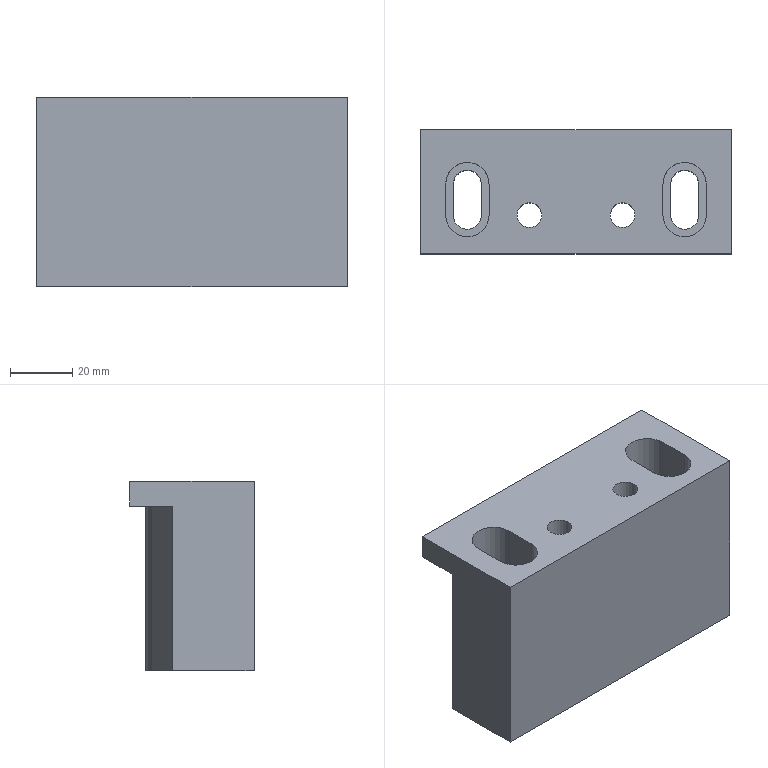Part | NX | features 1605158808 2 | 1 solid | 30 faces | box 100 x 40 x 61 mm | volume 179848 mm3 | plane 19 | cylinder 11 | commonest cylinder face diameters 9 x4 14 x4 8.001 x2 30 x1
STEP:
#1=CARTESIAN_POINT('',(-322.,-117.55,-2.5));
#2=VERTEX_POINT('',#1);
#3=CARTESIAN_POINT('',(-318.,-117.55,-2.5));
#4=DIRECTION('',(0.,0.,-1.));
#5=DIRECTION('',(-1.,0.,0.));
#6=AXIS2_PLACEMENT_3D('',#3,#4,#5);
#7=CIRCLE('',#6,4.);
#8=EDGE_CURVE('',#2,#2,#7,.T.);
#9=ORIENTED_EDGE('',*,*,#8,.F.);
#10=EDGE_LOOP('',(#9));
#11=FACE_BOUND('',#10,.T.);
#12=CARTESIAN_POINT('',(-352.,-117.55,-2.5));
#13=VERTEX_POINT('',#12);
#14=CARTESIAN_POINT('',(-348.,-117.55,-2.5));
#15=DIRECTION('',(0.,0.,-1.));
#16=DIRECTION('',(-1.,0.,0.));
#17=AXIS2_PLACEMENT_3D('',#14,#15,#16);
#18=CIRCLE('',#17,4.);
#19=EDGE_CURVE('',#13,#13,#18,.T.);
#20=ORIENTED_EDGE('',*,*,#19,.F.);
#21=EDGE_LOOP('',(#20));
#22=FACE_BOUND('',#21,.T.);
#23=CARTESIAN_POINT('',(-383.,-103.71,-2.5));
#24=VERTEX_POINT('',#23);
#25=CARTESIAN_POINT('',(-371.481,-97.06,-2.5));
#26=VERTEX_POINT('',#25);
#27=CARTESIAN_POINT('',(-349.761,-84.52,-2.5));
#28=DIRECTION('',(-0.866,-0.5,0.));
#29=VECTOR('',#28,1000.);
#30=LINE('',#27,#29);
#31=EDGE_CURVE('',#24,#26,#30,.F.);
#32=ORIENTED_EDGE('',*,*,#31,.T.);
#33=CARTESIAN_POINT('',(-363.981,-95.05,-2.5));
#34=VERTEX_POINT('',#33);
#35=CARTESIAN_POINT('',(-363.981,-110.05,-2.5));
#36=DIRECTION('',(0.,0.,-1.));
#37=DIRECTION('',(-1.,0.,0.));
#38=AXIS2_PLACEMENT_3D('',#35,#36,#37);
#39=CIRCLE('',#38,15.);
#40=EDGE_CURVE('',#26,#34,#39,.T.);
#41=ORIENTED_EDGE('',*,*,#40,.T.);
#42=CARTESIAN_POINT('',(-283.,-95.05,-2.5));
#43=VERTEX_POINT('',#42);
#44=CARTESIAN_POINT('',(-333.,-95.05,-2.5));
#45=DIRECTION('',(-1.,0.,0.));
#46=VECTOR('',#45,1000.);
#47=LINE('',#44,#46);
#48=EDGE_CURVE('',#43,#34,#47,.T.);
#49=ORIENTED_EDGE('',*,*,#48,.F.);
#50=CARTESIAN_POINT('',(-283.,-130.05,-2.5));
#51=VERTEX_POINT('',#50);
#52=CARTESIAN_POINT('',(-283.,7.95,-2.5));
#53=DIRECTION('',(0.,1.,0.));
#54=VECTOR('',#53,1000.);
#55=LINE('',#52,#54);
#56=EDGE_CURVE('',#51,#43,#55,.T.);
#57=ORIENTED_EDGE('',*,*,#56,.F.);
#58=CARTESIAN_POINT('',(-383.,-130.05,-2.5));
#59=VERTEX_POINT('',#58);
#60=CARTESIAN_POINT('',(-333.,-130.05,-2.5));
#61=DIRECTION('',(1.,0.,0.));
#62=VECTOR('',#61,1000.);
#63=LINE('',#60,#62);
#64=EDGE_CURVE('',#59,#51,#63,.T.);
#65=ORIENTED_EDGE('',*,*,#64,.F.);
#66=CARTESIAN_POINT('',(-383.,-113.55,-2.5));
#67=DIRECTION('',(0.,-1.,0.));
#68=VECTOR('',#67,1000.);
#69=LINE('',#66,#68);
#70=EDGE_CURVE('',#24,#59,#69,.T.);
#71=ORIENTED_EDGE('',*,*,#70,.F.);
#72=EDGE_LOOP('',(#32,#41,#49,#57,#65,#71));
#73=FACE_BOUND('',#72,.T.);
#74=CARTESIAN_POINT('',(-372.5,-107.55,-2.5));
#75=VERTEX_POINT('',#74);
#76=CARTESIAN_POINT('',(-363.5,-107.55,-2.5));
#77=VERTEX_POINT('',#76);
#78=CARTESIAN_POINT('',(-368.,-107.55,-2.5));
#79=DIRECTION('',(0.,0.,-1.));
#80=DIRECTION('',(-1.,0.,0.));
#81=AXIS2_PLACEMENT_3D('',#78,#79,#80);
#82=CIRCLE('',#81,4.5);
#83=EDGE_CURVE('',#75,#77,#82,.T.);
#84=ORIENTED_EDGE('',*,*,#83,.F.);
#85=CARTESIAN_POINT('',(-372.5,-117.55,-2.5));
#86=VERTEX_POINT('',#85);
#87=CARTESIAN_POINT('',(-372.5,-113.55,-2.5));
#88=DIRECTION('',(0.,1.,0.));
#89=VECTOR('',#88,1000.);
#90=LINE('',#87,#89);
#91=EDGE_CURVE('',#86,#75,#90,.T.);
#92=ORIENTED_EDGE('',*,*,#91,.F.);
#93=CARTESIAN_POINT('',(-363.5,-117.55,-2.5));
#94=VERTEX_POINT('',#93);
#95=CARTESIAN_POINT('',(-368.,-117.55,-2.5));
#96=DIRECTION('',(0.,0.,-1.));
#97=DIRECTION('',(-1.,0.,0.));
#98=AXIS2_PLACEMENT_3D('',#95,#96,#97);
#99=CIRCLE('',#98,4.5);
#100=EDGE_CURVE('',#94,#86,#99,.T.);
#101=ORIENTED_EDGE('',*,*,#100,.F.);
#102=CARTESIAN_POINT('',(-363.5,-113.55,-2.5));
#103=DIRECTION('',(0.,-1.,0.));
#104=VECTOR('',#103,1000.);
#105=LINE('',#102,#104);
#106=EDGE_CURVE('',#77,#94,#105,.T.);
#107=ORIENTED_EDGE('',*,*,#106,.F.);
#108=EDGE_LOOP('',(#84,#92,#101,#107));
#109=FACE_BOUND('',#108,.T.);
#110=CARTESIAN_POINT('',(-302.5,-107.55,-2.5));
#111=VERTEX_POINT('',#110);
#112=CARTESIAN_POINT('',(-293.5,-107.55,-2.5));
#113=VERTEX_POINT('',#112);
#114=CARTESIAN_POINT('',(-298.,-107.55,-2.5));
#115=DIRECTION('',(0.,0.,-1.));
#116=DIRECTION('',(-1.,0.,0.));
#117=AXIS2_PLACEMENT_3D('',#114,#115,#116);
#118=CIRCLE('',#117,4.5);
#119=EDGE_CURVE('',#111,#113,#118,.T.);
#120=ORIENTED_EDGE('',*,*,#119,.F.);
#121=CARTESIAN_POINT('',(-302.5,-117.55,-2.5));
#122=VERTEX_POINT('',#121);
#123=CARTESIAN_POINT('',(-302.5,-113.55,-2.5));
#124=DIRECTION('',(0.,1.,0.));
#125=VECTOR('',#124,1000.);
#126=LINE('',#123,#125);
#127=EDGE_CURVE('',#122,#111,#126,.T.);
#128=ORIENTED_EDGE('',*,*,#127,.F.);
#129=CARTESIAN_POINT('',(-293.5,-117.55,-2.5));
#130=VERTEX_POINT('',#129);
#131=CARTESIAN_POINT('',(-298.,-117.55,-2.5));
#132=DIRECTION('',(0.,0.,-1.));
#133=DIRECTION('',(-1.,0.,0.));
#134=AXIS2_PLACEMENT_3D('',#131,#132,#133);
#135=CIRCLE('',#134,4.5);
#136=EDGE_CURVE('',#130,#122,#135,.T.);
#137=ORIENTED_EDGE('',*,*,#136,.F.);
#138=CARTESIAN_POINT('',(-293.5,-113.55,-2.5));
#139=DIRECTION('',(0.,-1.,0.));
#140=VECTOR('',#139,1000.);
#141=LINE('',#138,#140);
#142=EDGE_CURVE('',#113,#130,#141,.T.);
#143=ORIENTED_EDGE('',*,*,#142,.F.);
#144=EDGE_LOOP('',(#120,#128,#137,#143));
#145=FACE_BOUND('',#144,.T.);
#146=CARTESIAN_POINT('',(-333.,-113.55,-2.5));
#147=DIRECTION('',(0.,0.,-1.));
#148=DIRECTION('',(-1.,0.,0.));
#149=AXIS2_PLACEMENT_3D('',#146,#147,#148);
#150=PLANE('',#149);
#151=ADVANCED_FACE('',(#11,#22,#73,#109,#145),#150,.T.);
#152=CARTESIAN_POINT('',(-361.,-117.55,58.5));
#153=VERTEX_POINT('',#152);
#154=CARTESIAN_POINT('',(-361.,-117.55,25.5));
#155=VERTEX_POINT('',#154);
#156=CARTESIAN_POINT('',(-361.,-117.55,-2.501));
#157=DIRECTION('',(0.,0.,1.));
#158=VECTOR('',#157,1000.);
#159=LINE('',#156,#158);
#160=EDGE_CURVE('',#153,#155,#159,.F.);
#161=ORIENTED_EDGE('',*,*,#160,.T.);
#162=CARTESIAN_POINT('',(-375.,-117.55,25.5));
#163=VERTEX_POINT('',#162);
#164=CARTESIAN_POINT('',(-368.,-117.55,25.5));
#165=DIRECTION('',(0.,0.,1.));
#166=DIRECTION('',(1.,0.,0.));
#167=AXIS2_PLACEMENT_3D('',#164,#165,#166);
#168=CIRCLE('',#167,7.);
#169=EDGE_CURVE('',#163,#155,#168,.T.);
#170=ORIENTED_EDGE('',*,*,#169,.F.);
#171=CARTESIAN_POINT('',(-375.,-117.55,58.5));
#172=VERTEX_POINT('',#171);
#173=CARTESIAN_POINT('',(-375.,-117.55,-2.501));
#174=DIRECTION('',(0.,0.,1.));
#175=VECTOR('',#174,1000.);
#176=LINE('',#173,#175);
#177=EDGE_CURVE('',#172,#163,#176,.F.);
#178=ORIENTED_EDGE('',*,*,#177,.F.);
#179=CARTESIAN_POINT('',(-368.,-117.55,58.5));
#180=DIRECTION('',(0.,0.,1.));
#181=DIRECTION('',(1.,0.,0.));
#182=AXIS2_PLACEMENT_3D('',#179,#180,#181);
#183=CIRCLE('',#182,7.);
#184=EDGE_CURVE('',#172,#153,#183,.T.);
#185=ORIENTED_EDGE('',*,*,#184,.T.);
#186=EDGE_LOOP('',(#161,#170,#178,#185));
#187=FACE_BOUND('',#186,.T.);
#188=CARTESIAN_POINT('',(-368.,-117.55,-2.501));
#189=DIRECTION('',(0.,0.,1.));
#190=DIRECTION('',(1.,0.,0.));
#191=AXIS2_PLACEMENT_3D('',#188,#189,#190);
#192=CYLINDRICAL_SURFACE('',#191,7.);
#193=ADVANCED_FACE('',(#187),#192,.F.);
#194=CARTESIAN_POINT('',(-363.981,-95.05,50.5));
#195=VERTEX_POINT('',#194);
#196=CARTESIAN_POINT('',(-283.,-95.05,50.5));
#197=VERTEX_POINT('',#196);
#198=CARTESIAN_POINT('',(-333.,-95.05,50.5));
#199=DIRECTION('',(1.,0.,0.));
#200=VECTOR('',#199,1000.);
#201=LINE('',#198,#200);
#202=EDGE_CURVE('',#195,#197,#201,.T.);
#203=ORIENTED_EDGE('',*,*,#202,.F.);
#204=CARTESIAN_POINT('',(-371.481,-97.06,50.5));
#205=VERTEX_POINT('',#204);
#206=CARTESIAN_POINT('',(-363.981,-110.05,50.5));
#207=DIRECTION('',(0.,0.,1.));
#208=DIRECTION('',(1.,0.,0.));
#209=AXIS2_PLACEMENT_3D('',#206,#207,#208);
#210=CIRCLE('',#209,15.);
#211=EDGE_CURVE('',#195,#205,#210,.T.);
#212=ORIENTED_EDGE('',*,*,#211,.T.);
#213=CARTESIAN_POINT('',(-383.,-103.71,50.5));
#214=VERTEX_POINT('',#213);
#215=CARTESIAN_POINT('',(-379.25,-101.545,50.5));
#216=DIRECTION('',(0.866,0.5,0.));
#217=VECTOR('',#216,1000.);
#218=LINE('',#215,#217);
#219=EDGE_CURVE('',#205,#214,#218,.F.);
#220=ORIENTED_EDGE('',*,*,#219,.T.);
#221=CARTESIAN_POINT('',(-383.,-90.05,50.5));
#222=VERTEX_POINT('',#221);
#223=CARTESIAN_POINT('',(-383.,-113.55,50.5));
#224=DIRECTION('',(0.,1.,0.));
#225=VECTOR('',#224,1000.);
#226=LINE('',#223,#225);
#227=EDGE_CURVE('',#214,#222,#226,.T.);
#228=ORIENTED_EDGE('',*,*,#227,.T.);
#229=CARTESIAN_POINT('',(-283.,-90.05,50.5));
#230=VERTEX_POINT('',#229);
#231=CARTESIAN_POINT('',(-333.,-90.05,50.5));
#232=DIRECTION('',(1.,0.,0.));
#233=VECTOR('',#232,1000.);
#234=LINE('',#231,#233);
#235=EDGE_CURVE('',#222,#230,#234,.T.);
#236=ORIENTED_EDGE('',*,*,#235,.T.);
#237=CARTESIAN_POINT('',(-283.,7.95,50.5));
#238=DIRECTION('',(0.,-1.,0.));
#239=VECTOR('',#238,1000.);
#240=LINE('',#237,#239);
#241=EDGE_CURVE('',#230,#197,#240,.T.);
#242=ORIENTED_EDGE('',*,*,#241,.T.);
#243=EDGE_LOOP('',(#203,#212,#220,#228,#236,#242));
#244=FACE_BOUND('',#243,.T.);
#245=CARTESIAN_POINT('',(-383.,-95.05,50.5));
#246=DIRECTION('',(0.,0.,1.));
#247=DIRECTION('',(1.,0.,0.));
#248=AXIS2_PLACEMENT_3D('',#245,#246,#247);
#249=PLANE('',#248);
#250=ADVANCED_FACE('',(#244),#249,.F.);
#251=CARTESIAN_POINT('',(-383.,-130.05,58.5));
#252=VERTEX_POINT('',#251);
#253=CARTESIAN_POINT('',(-383.,-130.05,-2.5));
#254=DIRECTION('',(0.,0.,1.));
#255=VECTOR('',#254,1000.);
#256=LINE('',#253,#255);
#257=EDGE_CURVE('',#59,#252,#256,.T.);
#258=ORIENTED_EDGE('',*,*,#257,.F.);
#259=ORIENTED_EDGE('',*,*,#64,.T.);
#260=CARTESIAN_POINT('',(-283.,-130.05,58.5));
#261=VERTEX_POINT('',#260);
#262=CARTESIAN_POINT('',(-283.,-130.05,-2.5));
#263=DIRECTION('',(0.,0.,1.));
#264=VECTOR('',#263,1000.);
#265=LINE('',#262,#264);
#266=EDGE_CURVE('',#51,#261,#265,.T.);
#267=ORIENTED_EDGE('',*,*,#266,.T.);
#268=CARTESIAN_POINT('',(-333.,-130.05,58.5));
#269=DIRECTION('',(-1.,0.,0.));
#270=VECTOR('',#269,1000.);
#271=LINE('',#268,#270);
#272=EDGE_CURVE('',#261,#252,#271,.T.);
#273=ORIENTED_EDGE('',*,*,#272,.T.);
#274=EDGE_LOOP('',(#258,#259,#267,#273));
#275=FACE_BOUND('',#274,.T.);
#276=CARTESIAN_POINT('',(-333.,-130.05,-2.5));
#277=DIRECTION('',(0.,-1.,0.));
#278=DIRECTION('',(0.,0.,-1.));
#279=AXIS2_PLACEMENT_3D('',#276,#277,#278);
#280=PLANE('',#279);
#281=ADVANCED_FACE('',(#275),#280,.T.);
#282=ORIENTED_EDGE('',*,*,#227,.F.);
#283=CARTESIAN_POINT('',(-383.,-103.71,-2.5));
#284=DIRECTION('',(0.,0.,-1.));
#285=VECTOR('',#284,1000.);
#286=LINE('',#283,#285);
#287=EDGE_CURVE('',#214,#24,#286,.T.);
#288=ORIENTED_EDGE('',*,*,#287,.T.);
#289=ORIENTED_EDGE('',*,*,#70,.T.);
#290=ORIENTED_EDGE('',*,*,#257,.T.);
#291=CARTESIAN_POINT('',(-383.,-90.05,58.5));
#292=VERTEX_POINT('',#291);
#293=CARTESIAN_POINT('',(-383.,-113.55,58.5));
#294=DIRECTION('',(0.,1.,0.));
#295=VECTOR('',#294,1000.);
#296=LINE('',#293,#295);
#297=EDGE_CURVE('',#252,#292,#296,.T.);
#298=ORIENTED_EDGE('',*,*,#297,.T.);
#299=CARTESIAN_POINT('',(-383.,-90.05,15.5));
#300=DIRECTION('',(0.,0.,1.));
#301=VECTOR('',#300,1000.);
#302=LINE('',#299,#301);
#303=EDGE_CURVE('',#222,#292,#302,.T.);
#304=ORIENTED_EDGE('',*,*,#303,.F.);
#305=EDGE_LOOP('',(#282,#288,#289,#290,#298,#304));
#306=FACE_BOUND('',#305,.T.);
#307=CARTESIAN_POINT('',(-383.,-113.55,-2.5));
#308=DIRECTION('',(-1.,0.,0.));
#309=DIRECTION('',(0.,0.,1.));
#310=AXIS2_PLACEMENT_3D('',#307,#308,#309);
#311=PLANE('',#310);
#312=ADVANCED_FACE('',(#306),#311,.T.);
#313=ORIENTED_EDGE('',*,*,#235,.F.);
#314=ORIENTED_EDGE('',*,*,#303,.T.);
#315=CARTESIAN_POINT('',(-283.,-90.05,58.5));
#316=VERTEX_POINT('',#315);
#317=CARTESIAN_POINT('',(-333.,-90.05,58.5));
#318=DIRECTION('',(1.,0.,0.));
#319=VECTOR('',#318,1000.);
#320=LINE('',#317,#319);
#321=EDGE_CURVE('',#292,#316,#320,.T.);
#322=ORIENTED_EDGE('',*,*,#321,.T.);
#323=CARTESIAN_POINT('',(-283.,-90.05,-17.5));
#324=DIRECTION('',(0.,0.,1.));
#325=VECTOR('',#324,1000.);
#326=LINE('',#323,#325);
#327=EDGE_CURVE('',#230,#316,#326,.T.);
#328=ORIENTED_EDGE('',*,*,#327,.F.);
#329=EDGE_LOOP('',(#313,#314,#322,#328));
#330=FACE_BOUND('',#329,.T.);
#331=CARTESIAN_POINT('',(-333.,-90.05,15.5));
#332=DIRECTION('',(0.,1.,0.));
#333=DIRECTION('',(0.,0.,1.));
#334=AXIS2_PLACEMENT_3D('',#331,#332,#333);
#335=PLANE('',#334);
#336=ADVANCED_FACE('',(#330),#335,.T.);
#337=ORIENTED_EDGE('',*,*,#241,.F.);
#338=ORIENTED_EDGE('',*,*,#327,.T.);
#339=CARTESIAN_POINT('',(-283.,7.95,58.5));
#340=DIRECTION('',(0.,-1.,0.));
#341=VECTOR('',#340,1000.);
#342=LINE('',#339,#341);
#343=EDGE_CURVE('',#316,#261,#342,.T.);
#344=ORIENTED_EDGE('',*,*,#343,.T.);
#345=ORIENTED_EDGE('',*,*,#266,.F.);
#346=ORIENTED_EDGE('',*,*,#56,.T.);
#347=CARTESIAN_POINT('',(-283.,-95.05,-35.5));
#348=DIRECTION('',(0.,0.,1.));
#349=VECTOR('',#348,1000.);
#350=LINE('',#347,#349);
#351=EDGE_CURVE('',#43,#197,#350,.T.);
#352=ORIENTED_EDGE('',*,*,#351,.T.);
#353=EDGE_LOOP('',(#337,#338,#344,#345,#346,#352));
#354=FACE_BOUND('',#353,.T.);
#355=CARTESIAN_POINT('',(-283.,7.95,-35.5));
#356=DIRECTION('',(1.,0.,0.));
#357=DIRECTION('',(0.,0.,-1.));
#358=AXIS2_PLACEMENT_3D('',#355,#356,#357);
#359=PLANE('',#358);
#360=ADVANCED_FACE('',(#354),#359,.T.);
#361=ORIENTED_EDGE('',*,*,#48,.T.);
#362=CARTESIAN_POINT('',(-363.981,-95.05,-2.5));
#363=DIRECTION('',(0.,0.,-1.));
#364=VECTOR('',#363,1000.);
#365=LINE('',#362,#364);
#366=EDGE_CURVE('',#34,#195,#365,.F.);
#367=ORIENTED_EDGE('',*,*,#366,.T.);
#368=ORIENTED_EDGE('',*,*,#202,.T.);
#369=ORIENTED_EDGE('',*,*,#351,.F.);
#370=EDGE_LOOP('',(#361,#367,#368,#369));
#371=FACE_BOUND('',#370,.T.);
#372=CARTESIAN_POINT('',(-333.,-95.05,-2.5));
#373=DIRECTION('',(0.,1.,0.));
#374=DIRECTION('',(0.,0.,1.));
#375=AXIS2_PLACEMENT_3D('',#372,#373,#374);
#376=PLANE('',#375);
#377=ADVANCED_FACE('',(#371),#376,.T.);
#378=ORIENTED_EDGE('',*,*,#219,.F.);
#379=CARTESIAN_POINT('',(-371.481,-97.06,-2.5));
#380=DIRECTION('',(0.,0.,1.));
#381=VECTOR('',#380,1000.);
#382=LINE('',#379,#381);
#383=EDGE_CURVE('',#205,#26,#382,.F.);
#384=ORIENTED_EDGE('',*,*,#383,.T.);
#385=ORIENTED_EDGE('',*,*,#31,.F.);
#386=ORIENTED_EDGE('',*,*,#287,.F.);
#387=EDGE_LOOP('',(#378,#384,#385,#386));
#388=FACE_BOUND('',#387,.T.);
#389=CARTESIAN_POINT('',(-368.,-95.05,-2.5));
#390=DIRECTION('',(0.5,-0.866,0.));
#391=DIRECTION('',(0.866,0.5,0.));
#392=AXIS2_PLACEMENT_3D('',#389,#390,#391);
#393=PLANE('',#392);
#394=ADVANCED_FACE('',(#388),#393,.F.);
#395=ORIENTED_EDGE('',*,*,#40,.F.);
#396=ORIENTED_EDGE('',*,*,#383,.F.);
#397=ORIENTED_EDGE('',*,*,#211,.F.);
#398=ORIENTED_EDGE('',*,*,#366,.F.);
#399=EDGE_LOOP('',(#395,#396,#397,#398));
#400=FACE_BOUND('',#399,.T.);
#401=CARTESIAN_POINT('',(-363.981,-110.05,-2.5));
#402=DIRECTION('',(0.,0.,-1.));
#403=DIRECTION('',(-1.,0.,0.));
#404=AXIS2_PLACEMENT_3D('',#401,#402,#403);
#405=CYLINDRICAL_SURFACE('',#404,15.);
#406=ADVANCED_FACE('',(#400),#405,.T.);
#407=ORIENTED_EDGE('',*,*,#177,.T.);
#408=CARTESIAN_POINT('',(-375.,-107.55,25.5));
#409=VERTEX_POINT('',#408);
#410=CARTESIAN_POINT('',(-375.,-113.55,25.5));
#411=DIRECTION('',(0.,-1.,0.));
#412=VECTOR('',#411,1000.);
#413=LINE('',#410,#412);
#414=EDGE_CURVE('',#409,#163,#413,.T.);
#415=ORIENTED_EDGE('',*,*,#414,.F.);
#416=CARTESIAN_POINT('',(-375.,-107.55,58.5));
#417=VERTEX_POINT('',#416);
#418=CARTESIAN_POINT('',(-375.,-107.55,-2.501));
#419=DIRECTION('',(0.,0.,1.));
#420=VECTOR('',#419,1000.);
#421=LINE('',#418,#420);
#422=EDGE_CURVE('',#409,#417,#421,.T.);
#423=ORIENTED_EDGE('',*,*,#422,.T.);
#424=CARTESIAN_POINT('',(-375.,-113.55,58.5));
#425=DIRECTION('',(0.,-1.,0.));
#426=VECTOR('',#425,1000.);
#427=LINE('',#424,#426);
#428=EDGE_CURVE('',#417,#172,#427,.T.);
#429=ORIENTED_EDGE('',*,*,#428,.T.);
#430=EDGE_LOOP('',(#407,#415,#423,#429));
#431=FACE_BOUND('',#430,.T.);
#432=CARTESIAN_POINT('',(-375.,-120.05,-2.501));
#433=DIRECTION('',(-1.,0.,0.));
#434=DIRECTION('',(0.,0.,1.));
#435=AXIS2_PLACEMENT_3D('',#432,#433,#434);
#436=PLANE('',#435);
#437=ADVANCED_FACE('',(#431),#436,.F.);
#438=CARTESIAN_POINT('',(-361.,-107.55,25.5));
#439=VERTEX_POINT('',#438);
#440=CARTESIAN_POINT('',(-361.,-107.55,58.5));
#441=VERTEX_POINT('',#440);
#442=CARTESIAN_POINT('',(-361.,-107.55,-2.501));
#443=DIRECTION('',(0.,0.,1.));
#444=VECTOR('',#443,1000.);
#445=LINE('',#442,#444);
#446=EDGE_CURVE('',#439,#441,#445,.T.);
#447=ORIENTED_EDGE('',*,*,#446,.F.);
#448=CARTESIAN_POINT('',(-361.,-113.55,25.5));
#449=DIRECTION('',(0.,1.,0.));
#450=VECTOR('',#449,1000.);
#451=LINE('',#448,#450);
#452=EDGE_CURVE('',#155,#439,#451,.T.);
#453=ORIENTED_EDGE('',*,*,#452,.F.);
#454=ORIENTED_EDGE('',*,*,#160,.F.);
#455=CARTESIAN_POINT('',(-361.,-113.55,58.5));
#456=DIRECTION('',(0.,1.,0.));
#457=VECTOR('',#456,1000.);
#458=LINE('',#455,#457);
#459=EDGE_CURVE('',#153,#441,#458,.T.);
#460=ORIENTED_EDGE('',*,*,#459,.T.);
#461=EDGE_LOOP('',(#447,#453,#454,#460));
#462=FACE_BOUND('',#461,.T.);
#463=CARTESIAN_POINT('',(-361.,-105.05,-2.501));
#464=DIRECTION('',(1.,0.,0.));
#465=DIRECTION('',(0.,0.,-1.));
#466=AXIS2_PLACEMENT_3D('',#463,#464,#465);
#467=PLANE('',#466);
#468=ADVANCED_FACE('',(#462),#467,.F.);
#469=ORIENTED_EDGE('',*,*,#422,.F.);
#470=CARTESIAN_POINT('',(-368.,-107.55,25.5));
#471=DIRECTION('',(0.,0.,1.));
#472=DIRECTION('',(1.,0.,0.));
#473=AXIS2_PLACEMENT_3D('',#470,#471,#472);
#474=CIRCLE('',#473,7.);
#475=EDGE_CURVE('',#439,#409,#474,.T.);
#476=ORIENTED_EDGE('',*,*,#475,.F.);
#477=ORIENTED_EDGE('',*,*,#446,.T.);
#478=CARTESIAN_POINT('',(-368.,-107.55,58.5));
#479=DIRECTION('',(0.,0.,1.));
#480=DIRECTION('',(1.,0.,0.));
#481=AXIS2_PLACEMENT_3D('',#478,#479,#480);
#482=CIRCLE('',#481,7.);
#483=EDGE_CURVE('',#441,#417,#482,.T.);
#484=ORIENTED_EDGE('',*,*,#483,.T.);
#485=EDGE_LOOP('',(#469,#476,#477,#484));
#486=FACE_BOUND('',#485,.T.);
#487=CARTESIAN_POINT('',(-368.,-107.55,-2.501));
#488=DIRECTION('',(0.,0.,1.));
#489=DIRECTION('',(1.,0.,0.));
#490=AXIS2_PLACEMENT_3D('',#487,#488,#489);
#491=CYLINDRICAL_SURFACE('',#490,7.);
#492=ADVANCED_FACE('',(#486),#491,.F.);
#493=CARTESIAN_POINT('',(-363.5,-107.55,25.5));
#494=VERTEX_POINT('',#493);
#495=CARTESIAN_POINT('',(-372.5,-107.55,25.5));
#496=VERTEX_POINT('',#495);
#497=CARTESIAN_POINT('',(-368.,-107.55,25.5));
#498=DIRECTION('',(0.,0.,1.));
#499=DIRECTION('',(1.,0.,0.));
#500=AXIS2_PLACEMENT_3D('',#497,#498,#499);
#501=CIRCLE('',#500,4.5);
#502=EDGE_CURVE('',#494,#496,#501,.T.);
#503=ORIENTED_EDGE('',*,*,#502,.T.);
#504=CARTESIAN_POINT('',(-372.5,-107.55,-2.501));
#505=DIRECTION('',(0.,0.,1.));
#506=VECTOR('',#505,1000.);
#507=LINE('',#504,#506);
#508=EDGE_CURVE('',#75,#496,#507,.T.);
#509=ORIENTED_EDGE('',*,*,#508,.F.);
#510=ORIENTED_EDGE('',*,*,#83,.T.);
#511=CARTESIAN_POINT('',(-363.5,-107.55,-2.501));
#512=DIRECTION('',(0.,0.,1.));
#513=VECTOR('',#512,1000.);
#514=LINE('',#511,#513);
#515=EDGE_CURVE('',#77,#494,#514,.T.);
#516=ORIENTED_EDGE('',*,*,#515,.T.);
#517=EDGE_LOOP('',(#503,#509,#510,#516));
#518=FACE_BOUND('',#517,.T.);
#519=CARTESIAN_POINT('',(-368.,-107.55,-2.501));
#520=DIRECTION('',(0.,0.,1.));
#521=DIRECTION('',(1.,0.,0.));
#522=AXIS2_PLACEMENT_3D('',#519,#520,#521);
#523=CYLINDRICAL_SURFACE('',#522,4.5);
#524=ADVANCED_FACE('',(#518),#523,.F.);
#525=ORIENTED_EDGE('',*,*,#502,.F.);
#526=CARTESIAN_POINT('',(-363.5,-117.55,25.5));
#527=VERTEX_POINT('',#526);
#528=CARTESIAN_POINT('',(-363.5,-113.55,25.5));
#529=DIRECTION('',(0.,1.,0.));
#530=VECTOR('',#529,1000.);
#531=LINE('',#528,#530);
#532=EDGE_CURVE('',#527,#494,#531,.T.);
#533=ORIENTED_EDGE('',*,*,#532,.F.);
#534=CARTESIAN_POINT('',(-372.5,-117.55,25.5));
#535=VERTEX_POINT('',#534);
#536=CARTESIAN_POINT('',(-368.,-117.55,25.5));
#537=DIRECTION('',(0.,0.,1.));
#538=DIRECTION('',(1.,0.,0.));
#539=AXIS2_PLACEMENT_3D('',#536,#537,#538);
#540=CIRCLE('',#539,4.5);
#541=EDGE_CURVE('',#535,#527,#540,.T.);
#542=ORIENTED_EDGE('',*,*,#541,.F.);
#543=CARTESIAN_POINT('',(-372.5,-113.55,25.5));
#544=DIRECTION('',(0.,-1.,0.));
#545=VECTOR('',#544,1000.);
#546=LINE('',#543,#545);
#547=EDGE_CURVE('',#496,#535,#546,.T.);
#548=ORIENTED_EDGE('',*,*,#547,.F.);
#549=EDGE_LOOP('',(#525,#533,#542,#548));
#550=FACE_BOUND('',#549,.T.);
#551=ORIENTED_EDGE('',*,*,#169,.T.);
#552=ORIENTED_EDGE('',*,*,#452,.T.);
#553=ORIENTED_EDGE('',*,*,#475,.T.);
#554=ORIENTED_EDGE('',*,*,#414,.T.);
#555=EDGE_LOOP('',(#551,#552,#553,#554));
#556=FACE_BOUND('',#555,.T.);
#557=CARTESIAN_POINT('',(-333.,-113.55,25.5));
#558=DIRECTION('',(0.,0.,1.));
#559=DIRECTION('',(1.,0.,0.));
#560=AXIS2_PLACEMENT_3D('',#557,#558,#559);
#561=PLANE('',#560);
#562=ADVANCED_FACE('',(#550,#556),#561,.T.);
#563=ORIENTED_EDGE('',*,*,#547,.T.);
#564=CARTESIAN_POINT('',(-372.5,-117.55,-2.501));
#565=DIRECTION('',(0.,0.,1.));
#566=VECTOR('',#565,1000.);
#567=LINE('',#564,#566);
#568=EDGE_CURVE('',#86,#535,#567,.T.);
#569=ORIENTED_EDGE('',*,*,#568,.F.);
#570=ORIENTED_EDGE('',*,*,#91,.T.);
#571=ORIENTED_EDGE('',*,*,#508,.T.);
#572=EDGE_LOOP('',(#563,#569,#570,#571));
#573=FACE_BOUND('',#572,.T.);
#574=CARTESIAN_POINT('',(-372.5,-120.05,-2.501));
#575=DIRECTION('',(-1.,0.,0.));
#576=DIRECTION('',(0.,0.,1.));
#577=AXIS2_PLACEMENT_3D('',#574,#575,#576);
#578=PLANE('',#577);
#579=ADVANCED_FACE('',(#573),#578,.F.);
#580=ORIENTED_EDGE('',*,*,#100,.T.);
#581=ORIENTED_EDGE('',*,*,#568,.T.);
#582=ORIENTED_EDGE('',*,*,#541,.T.);
#583=CARTESIAN_POINT('',(-363.5,-117.55,-2.501));
#584=DIRECTION('',(0.,0.,1.));
#585=VECTOR('',#584,1000.);
#586=LINE('',#583,#585);
#587=EDGE_CURVE('',#94,#527,#586,.T.);
#588=ORIENTED_EDGE('',*,*,#587,.F.);
#589=EDGE_LOOP('',(#580,#581,#582,#588));
#590=FACE_BOUND('',#589,.T.);
#591=CARTESIAN_POINT('',(-368.,-117.55,-2.501));
#592=DIRECTION('',(0.,0.,1.));
#593=DIRECTION('',(1.,0.,0.));
#594=AXIS2_PLACEMENT_3D('',#591,#592,#593);
#595=CYLINDRICAL_SURFACE('',#594,4.5);
#596=ADVANCED_FACE('',(#590),#595,.F.);
#597=ORIENTED_EDGE('',*,*,#532,.T.);
#598=ORIENTED_EDGE('',*,*,#515,.F.);
#599=ORIENTED_EDGE('',*,*,#106,.T.);
#600=ORIENTED_EDGE('',*,*,#587,.T.);
#601=EDGE_LOOP('',(#597,#598,#599,#600));
#602=FACE_BOUND('',#601,.T.);
#603=CARTESIAN_POINT('',(-363.5,-105.05,-2.501));
#604=DIRECTION('',(1.,0.,0.));
#605=DIRECTION('',(0.,0.,-1.));
#606=AXIS2_PLACEMENT_3D('',#603,#604,#605);
#607=PLANE('',#606);
#608=ADVANCED_FACE('',(#602),#607,.F.);
#609=CARTESIAN_POINT('',(-291.,-117.55,25.5));
#610=VERTEX_POINT('',#609);
#611=CARTESIAN_POINT('',(-305.,-117.55,25.5));
#612=VERTEX_POINT('',#611);
#613=CARTESIAN_POINT('',(-298.,-117.55,25.5));
#614=DIRECTION('',(0.,0.,1.));
#615=DIRECTION('',(1.,0.,0.));
#616=AXIS2_PLACEMENT_3D('',#613,#614,#615);
#617=CIRCLE('',#616,7.);
#618=EDGE_CURVE('',#610,#612,#617,.F.);
#619=ORIENTED_EDGE('',*,*,#618,.T.);
#620=CARTESIAN_POINT('',(-305.,-117.55,58.5));
#621=VERTEX_POINT('',#620);
#622=CARTESIAN_POINT('',(-305.,-117.55,-2.501));
#623=DIRECTION('',(0.,0.,1.));
#624=VECTOR('',#623,1000.);
#625=LINE('',#622,#624);
#626=EDGE_CURVE('',#612,#621,#625,.T.);
#627=ORIENTED_EDGE('',*,*,#626,.T.);
#628=CARTESIAN_POINT('',(-291.,-117.55,58.5));
#629=VERTEX_POINT('',#628);
#630=CARTESIAN_POINT('',(-298.,-117.55,58.5));
#631=DIRECTION('',(0.,0.,1.));
#632=DIRECTION('',(1.,0.,0.));
#633=AXIS2_PLACEMENT_3D('',#630,#631,#632);
#634=CIRCLE('',#633,7.);
#635=EDGE_CURVE('',#629,#621,#634,.F.);
#636=ORIENTED_EDGE('',*,*,#635,.F.);
#637=CARTESIAN_POINT('',(-291.,-117.55,-2.501));
#638=DIRECTION('',(0.,0.,1.));
#639=VECTOR('',#638,1000.);
#640=LINE('',#637,#639);
#641=EDGE_CURVE('',#610,#629,#640,.T.);
#642=ORIENTED_EDGE('',*,*,#641,.F.);
#643=EDGE_LOOP('',(#619,#627,#636,#642));
#644=FACE_BOUND('',#643,.T.);
#645=CARTESIAN_POINT('',(-298.,-117.55,-2.501));
#646=DIRECTION('',(0.,0.,1.));
#647=DIRECTION('',(1.,0.,0.));
#648=AXIS2_PLACEMENT_3D('',#645,#646,#647);
#649=CYLINDRICAL_SURFACE('',#648,7.);
#650=ADVANCED_FACE('',(#644),#649,.F.);
#651=CARTESIAN_POINT('',(-305.,-107.55,25.5));
#652=VERTEX_POINT('',#651);
#653=CARTESIAN_POINT('',(-305.,-113.55,25.5));
#654=DIRECTION('',(0.,1.,0.));
#655=VECTOR('',#654,1000.);
#656=LINE('',#653,#655);
#657=EDGE_CURVE('',#612,#652,#656,.T.);
#658=ORIENTED_EDGE('',*,*,#657,.T.);
#659=CARTESIAN_POINT('',(-305.,-107.55,58.5));
#660=VERTEX_POINT('',#659);
#661=CARTESIAN_POINT('',(-305.,-107.55,-2.501));
#662=DIRECTION('',(0.,0.,1.));
#663=VECTOR('',#662,1000.);
#664=LINE('',#661,#663);
#665=EDGE_CURVE('',#652,#660,#664,.T.);
#666=ORIENTED_EDGE('',*,*,#665,.T.);
#667=CARTESIAN_POINT('',(-305.,-113.55,58.5));
#668=DIRECTION('',(0.,1.,0.));
#669=VECTOR('',#668,1000.);
#670=LINE('',#667,#669);
#671=EDGE_CURVE('',#621,#660,#670,.T.);
#672=ORIENTED_EDGE('',*,*,#671,.F.);
#673=ORIENTED_EDGE('',*,*,#626,.F.);
#674=EDGE_LOOP('',(#658,#666,#672,#673));
#675=FACE_BOUND('',#674,.T.);
#676=CARTESIAN_POINT('',(-305.,-107.55,-2.501));
#677=DIRECTION('',(1.,0.,0.));
#678=DIRECTION('',(0.,0.,-1.));
#679=AXIS2_PLACEMENT_3D('',#676,#677,#678);
#680=PLANE('',#679);
#681=ADVANCED_FACE('',(#675),#680,.T.);
#682=CARTESIAN_POINT('',(-291.,-107.55,25.5));
#683=VERTEX_POINT('',#682);
#684=CARTESIAN_POINT('',(-298.,-107.55,25.5));
#685=DIRECTION('',(0.,0.,1.));
#686=DIRECTION('',(1.,0.,0.));
#687=AXIS2_PLACEMENT_3D('',#684,#685,#686);
#688=CIRCLE('',#687,7.);
#689=EDGE_CURVE('',#652,#683,#688,.F.);
#690=ORIENTED_EDGE('',*,*,#689,.T.);
#691=CARTESIAN_POINT('',(-291.,-107.55,58.5));
#692=VERTEX_POINT('',#691);
#693=CARTESIAN_POINT('',(-291.,-107.55,-2.501));
#694=DIRECTION('',(0.,0.,1.));
#695=VECTOR('',#694,1000.);
#696=LINE('',#693,#695);
#697=EDGE_CURVE('',#683,#692,#696,.T.);
#698=ORIENTED_EDGE('',*,*,#697,.T.);
#699=CARTESIAN_POINT('',(-298.,-107.55,58.5));
#700=DIRECTION('',(0.,0.,1.));
#701=DIRECTION('',(1.,0.,0.));
#702=AXIS2_PLACEMENT_3D('',#699,#700,#701);
#703=CIRCLE('',#702,7.);
#704=EDGE_CURVE('',#660,#692,#703,.F.);
#705=ORIENTED_EDGE('',*,*,#704,.F.);
#706=ORIENTED_EDGE('',*,*,#665,.F.);
#707=EDGE_LOOP('',(#690,#698,#705,#706));
#708=FACE_BOUND('',#707,.T.);
#709=CARTESIAN_POINT('',(-298.,-107.55,-2.501));
#710=DIRECTION('',(0.,0.,1.));
#711=DIRECTION('',(1.,0.,0.));
#712=AXIS2_PLACEMENT_3D('',#709,#710,#711);
#713=CYLINDRICAL_SURFACE('',#712,7.);
#714=ADVANCED_FACE('',(#708),#713,.F.);
#715=CARTESIAN_POINT('',(-291.,-113.55,25.5));
#716=DIRECTION('',(0.,-1.,0.));
#717=VECTOR('',#716,1000.);
#718=LINE('',#715,#717);
#719=EDGE_CURVE('',#683,#610,#718,.T.);
#720=ORIENTED_EDGE('',*,*,#719,.T.);
#721=ORIENTED_EDGE('',*,*,#641,.T.);
#722=CARTESIAN_POINT('',(-291.,-113.55,58.5));
#723=DIRECTION('',(0.,-1.,0.));
#724=VECTOR('',#723,1000.);
#725=LINE('',#722,#724);
#726=EDGE_CURVE('',#692,#629,#725,.T.);
#727=ORIENTED_EDGE('',*,*,#726,.F.);
#728=ORIENTED_EDGE('',*,*,#697,.F.);
#729=EDGE_LOOP('',(#720,#721,#727,#728));
#730=FACE_BOUND('',#729,.T.);
#731=CARTESIAN_POINT('',(-291.,-117.55,-2.501));
#732=DIRECTION('',(-1.,0.,0.));
#733=DIRECTION('',(0.,0.,1.));
#734=AXIS2_PLACEMENT_3D('',#731,#732,#733);
#735=PLANE('',#734);
#736=ADVANCED_FACE('',(#730),#735,.T.);
#737=CARTESIAN_POINT('',(-293.5,-117.55,25.5));
#738=VERTEX_POINT('',#737);
#739=CARTESIAN_POINT('',(-293.5,-107.55,25.5));
#740=VERTEX_POINT('',#739);
#741=CARTESIAN_POINT('',(-293.5,-113.55,25.5));
#742=DIRECTION('',(0.,1.,0.));
#743=VECTOR('',#742,1000.);
#744=LINE('',#741,#743);
#745=EDGE_CURVE('',#738,#740,#744,.T.);
#746=ORIENTED_EDGE('',*,*,#745,.T.);
#747=CARTESIAN_POINT('',(-293.5,-107.55,-2.501));
#748=DIRECTION('',(0.,0.,1.));
#749=VECTOR('',#748,1000.);
#750=LINE('',#747,#749);
#751=EDGE_CURVE('',#113,#740,#750,.T.);
#752=ORIENTED_EDGE('',*,*,#751,.F.);
#753=ORIENTED_EDGE('',*,*,#142,.T.);
#754=CARTESIAN_POINT('',(-293.5,-117.55,-2.501));
#755=DIRECTION('',(0.,0.,1.));
#756=VECTOR('',#755,1000.);
#757=LINE('',#754,#756);
#758=EDGE_CURVE('',#130,#738,#757,.T.);
#759=ORIENTED_EDGE('',*,*,#758,.T.);
#760=EDGE_LOOP('',(#746,#752,#753,#759));
#761=FACE_BOUND('',#760,.T.);
#762=CARTESIAN_POINT('',(-293.5,-107.55,-2.501));
#763=DIRECTION('',(1.,0.,0.));
#764=DIRECTION('',(0.,0.,-1.));
#765=AXIS2_PLACEMENT_3D('',#762,#763,#764);
#766=PLANE('',#765);
#767=ADVANCED_FACE('',(#761),#766,.F.);
#768=CARTESIAN_POINT('',(-302.5,-117.55,25.5));
#769=VERTEX_POINT('',#768);
#770=CARTESIAN_POINT('',(-298.,-117.55,25.5));
#771=DIRECTION('',(0.,0.,1.));
#772=DIRECTION('',(1.,0.,0.));
#773=AXIS2_PLACEMENT_3D('',#770,#771,#772);
#774=CIRCLE('',#773,4.5);
#775=EDGE_CURVE('',#769,#738,#774,.T.);
#776=ORIENTED_EDGE('',*,*,#775,.T.);
#777=ORIENTED_EDGE('',*,*,#758,.F.);
#778=ORIENTED_EDGE('',*,*,#136,.T.);
#779=CARTESIAN_POINT('',(-302.5,-117.55,-2.501));
#780=DIRECTION('',(0.,0.,1.));
#781=VECTOR('',#780,1000.);
#782=LINE('',#779,#781);
#783=EDGE_CURVE('',#122,#769,#782,.T.);
#784=ORIENTED_EDGE('',*,*,#783,.T.);
#785=EDGE_LOOP('',(#776,#777,#778,#784));
#786=FACE_BOUND('',#785,.T.);
#787=CARTESIAN_POINT('',(-298.,-117.55,-2.501));
#788=DIRECTION('',(0.,0.,1.));
#789=DIRECTION('',(1.,0.,0.));
#790=AXIS2_PLACEMENT_3D('',#787,#788,#789);
#791=CYLINDRICAL_SURFACE('',#790,4.5);
#792=ADVANCED_FACE('',(#786),#791,.F.);
#793=CARTESIAN_POINT('',(-302.5,-107.55,25.5));
#794=VERTEX_POINT('',#793);
#795=CARTESIAN_POINT('',(-302.5,-113.55,25.5));
#796=DIRECTION('',(0.,-1.,0.));
#797=VECTOR('',#796,1000.);
#798=LINE('',#795,#797);
#799=EDGE_CURVE('',#794,#769,#798,.T.);
#800=ORIENTED_EDGE('',*,*,#799,.T.);
#801=ORIENTED_EDGE('',*,*,#783,.F.);
#802=ORIENTED_EDGE('',*,*,#127,.T.);
#803=CARTESIAN_POINT('',(-302.5,-107.55,-2.501));
#804=DIRECTION('',(0.,0.,1.));
#805=VECTOR('',#804,1000.);
#806=LINE('',#803,#805);
#807=EDGE_CURVE('',#111,#794,#806,.T.);
#808=ORIENTED_EDGE('',*,*,#807,.T.);
#809=EDGE_LOOP('',(#800,#801,#802,#808));
#810=FACE_BOUND('',#809,.T.);
#811=CARTESIAN_POINT('',(-302.5,-117.55,-2.501));
#812=DIRECTION('',(-1.,0.,0.));
#813=DIRECTION('',(0.,0.,1.));
#814=AXIS2_PLACEMENT_3D('',#811,#812,#813);
#815=PLANE('',#814);
#816=ADVANCED_FACE('',(#810),#815,.F.);
#817=ORIENTED_EDGE('',*,*,#618,.F.);
#818=ORIENTED_EDGE('',*,*,#719,.F.);
#819=ORIENTED_EDGE('',*,*,#689,.F.);
#820=ORIENTED_EDGE('',*,*,#657,.F.);
#821=EDGE_LOOP('',(#817,#818,#819,#820));
#822=FACE_BOUND('',#821,.T.);
#823=CARTESIAN_POINT('',(-298.,-107.55,25.5));
#824=DIRECTION('',(0.,0.,1.));
#825=DIRECTION('',(1.,0.,0.));
#826=AXIS2_PLACEMENT_3D('',#823,#824,#825);
#827=CIRCLE('',#826,4.5);
#828=EDGE_CURVE('',#740,#794,#827,.T.);
#829=ORIENTED_EDGE('',*,*,#828,.F.);
#830=ORIENTED_EDGE('',*,*,#745,.F.);
#831=ORIENTED_EDGE('',*,*,#775,.F.);
#832=ORIENTED_EDGE('',*,*,#799,.F.);
#833=EDGE_LOOP('',(#829,#830,#831,#832));
#834=FACE_BOUND('',#833,.T.);
#835=CARTESIAN_POINT('',(-333.,-113.55,25.5));
#836=DIRECTION('',(0.,0.,1.));
#837=DIRECTION('',(1.,0.,0.));
#838=AXIS2_PLACEMENT_3D('',#835,#836,#837);
#839=PLANE('',#838);
#840=ADVANCED_FACE('',(#822,#834),#839,.T.);
#841=ORIENTED_EDGE('',*,*,#828,.T.);
#842=ORIENTED_EDGE('',*,*,#807,.F.);
#843=ORIENTED_EDGE('',*,*,#119,.T.);
#844=ORIENTED_EDGE('',*,*,#751,.T.);
#845=EDGE_LOOP('',(#841,#842,#843,#844));
#846=FACE_BOUND('',#845,.T.);
#847=CARTESIAN_POINT('',(-298.,-107.55,-2.501));
#848=DIRECTION('',(0.,0.,1.));
#849=DIRECTION('',(1.,0.,0.));
#850=AXIS2_PLACEMENT_3D('',#847,#848,#849);
#851=CYLINDRICAL_SURFACE('',#850,4.5);
#852=ADVANCED_FACE('',(#846),#851,.F.);
#853=CARTESIAN_POINT('',(-344.,-117.55,58.5));
#854=VERTEX_POINT('',#853);
#855=CARTESIAN_POINT('',(-348.,-117.55,58.5));
#856=DIRECTION('',(0.,0.,1.));
#857=DIRECTION('',(1.,0.,0.));
#858=AXIS2_PLACEMENT_3D('',#855,#856,#857);
#859=CIRCLE('',#858,4.);
#860=EDGE_CURVE('',#854,#854,#859,.T.);
#861=ORIENTED_EDGE('',*,*,#860,.T.);
#862=EDGE_LOOP('',(#861));
#863=FACE_BOUND('',#862,.T.);
#864=ORIENTED_EDGE('',*,*,#19,.T.);
#865=EDGE_LOOP('',(#864));
#866=FACE_BOUND('',#865,.T.);
#867=CARTESIAN_POINT('',(-348.,-117.55,-2.501));
#868=DIRECTION('',(0.,0.,1.));
#869=DIRECTION('',(1.,0.,0.));
#870=AXIS2_PLACEMENT_3D('',#867,#868,#869);
#871=CYLINDRICAL_SURFACE('',#870,4.);
#872=ADVANCED_FACE('',(#863,#866),#871,.F.);
#873=CARTESIAN_POINT('',(-314.,-117.55,58.5));
#874=VERTEX_POINT('',#873);
#875=CARTESIAN_POINT('',(-318.,-117.55,58.5));
#876=DIRECTION('',(0.,0.,1.));
#877=DIRECTION('',(1.,0.,0.));
#878=AXIS2_PLACEMENT_3D('',#875,#876,#877);
#879=CIRCLE('',#878,4.);
#880=EDGE_CURVE('',#874,#874,#879,.T.);
#881=ORIENTED_EDGE('',*,*,#880,.T.);
#882=EDGE_LOOP('',(#881));
#883=FACE_BOUND('',#882,.T.);
#884=ORIENTED_EDGE('',*,*,#8,.T.);
#885=EDGE_LOOP('',(#884));
#886=FACE_BOUND('',#885,.T.);
#887=CARTESIAN_POINT('',(-318.,-117.55,-2.501));
#888=DIRECTION('',(0.,0.,1.));
#889=DIRECTION('',(1.,0.,0.));
#890=AXIS2_PLACEMENT_3D('',#887,#888,#889);
#891=CYLINDRICAL_SURFACE('',#890,4.);
#892=ADVANCED_FACE('',(#883,#886),#891,.F.);
#893=ORIENTED_EDGE('',*,*,#726,.T.);
#894=ORIENTED_EDGE('',*,*,#635,.T.);
#895=ORIENTED_EDGE('',*,*,#671,.T.);
#896=ORIENTED_EDGE('',*,*,#704,.T.);
#897=EDGE_LOOP('',(#893,#894,#895,#896));
#898=FACE_BOUND('',#897,.T.);
#899=ORIENTED_EDGE('',*,*,#483,.F.);
#900=ORIENTED_EDGE('',*,*,#459,.F.);
#901=ORIENTED_EDGE('',*,*,#184,.F.);
#902=ORIENTED_EDGE('',*,*,#428,.F.);
#903=EDGE_LOOP('',(#899,#900,#901,#902));
#904=FACE_BOUND('',#903,.T.);
#905=ORIENTED_EDGE('',*,*,#272,.F.);
#906=ORIENTED_EDGE('',*,*,#343,.F.);
#907=ORIENTED_EDGE('',*,*,#321,.F.);
#908=ORIENTED_EDGE('',*,*,#297,.F.);
#909=EDGE_LOOP('',(#905,#906,#907,#908));
#910=FACE_BOUND('',#909,.T.);
#911=ORIENTED_EDGE('',*,*,#860,.F.);
#912=EDGE_LOOP('',(#911));
#913=FACE_BOUND('',#912,.T.);
#914=ORIENTED_EDGE('',*,*,#880,.F.);
#915=EDGE_LOOP('',(#914));
#916=FACE_BOUND('',#915,.T.);
#917=CARTESIAN_POINT('',(-333.,-113.55,58.5));
#918=DIRECTION('',(0.,0.,1.));
#919=DIRECTION('',(1.,0.,0.));
#920=AXIS2_PLACEMENT_3D('',#917,#918,#919);
#921=PLANE('',#920);
#922=ADVANCED_FACE('',(#898,#904,#910,#913,#916),#921,.T.);
#923=CLOSED_SHELL('',(#151,#193,#250,#281,#312,#336,#360,#377,#394,#406,#437,#468,#492,#524,#562,#579,#596,#608,#650,#681,#714,#736,#767,#792,#816,#840,#852,#872,#892,#922));
#924=MANIFOLD_SOLID_BREP('',#923);
#925=(LENGTH_UNIT()NAMED_UNIT(*)SI_UNIT(.MILLI.,.METRE.));
#926=UNCERTAINTY_MEASURE_WITH_UNIT(LENGTH_MEASURE(0.00001),#925,'','');
#927=(NAMED_UNIT(*)PLANE_ANGLE_UNIT()SI_UNIT($,.RADIAN.));
#928=(NAMED_UNIT(*)SI_UNIT($,.STERADIAN.)SOLID_ANGLE_UNIT());
#929=(GEOMETRIC_REPRESENTATION_CONTEXT(3)GLOBAL_UNCERTAINTY_ASSIGNED_CONTEXT((#926))GLOBAL_UNIT_ASSIGNED_CONTEXT((#925,#927,#928))REPRESENTATION_CONTEXT('',''));
#930=ADVANCED_BREP_SHAPE_REPRESENTATION('',(#924),#929);